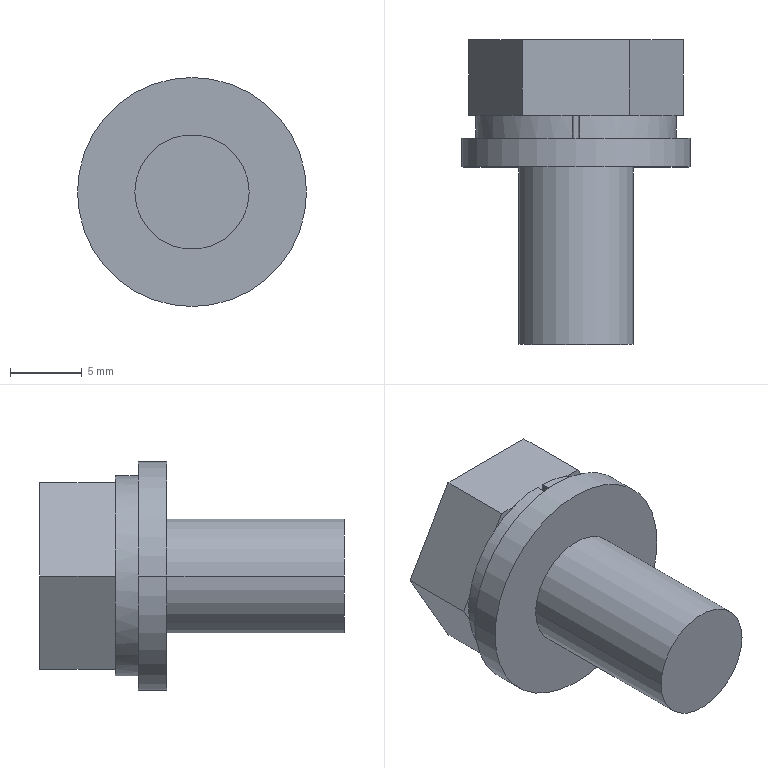Part | STEP file | LIB_36623152_M8X16 | 1 solid | 32 faces | box 16 x 21.3 x 16 mm | volume 2046 mm3 | plane 26 | cylinder 6 | commonest cylinder face diameters 8 x3 16 x2 14 x1